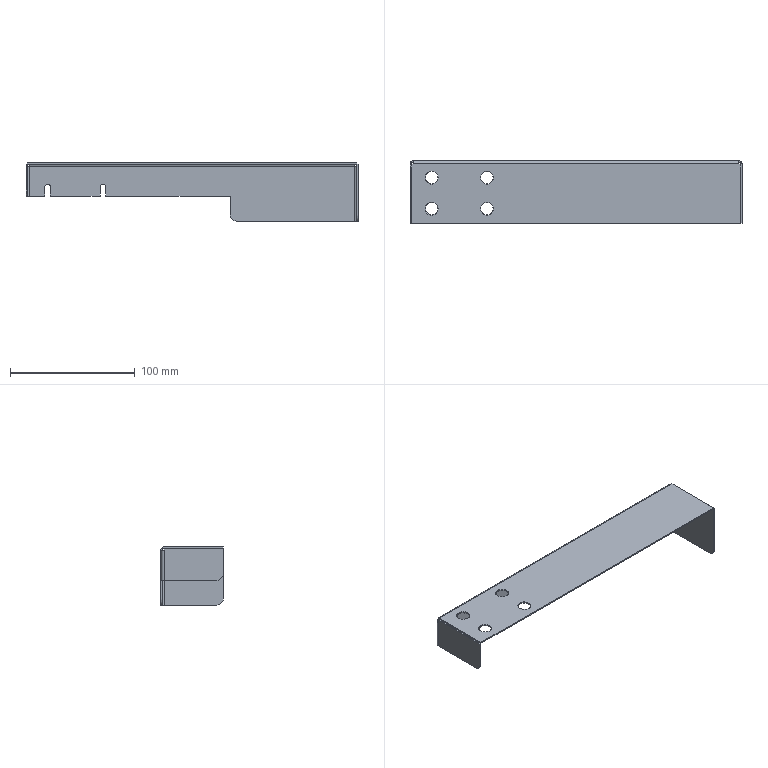Part | NX | 1 solid | 59 faces | box 266 x 50 x 46.7 mm | volume 24838 mm3 | plane 32 | cylinder 19 | cone 8 | commonest cylinder face diameters 10 x11 3.2 x3 5.2 x3 4.5 x2